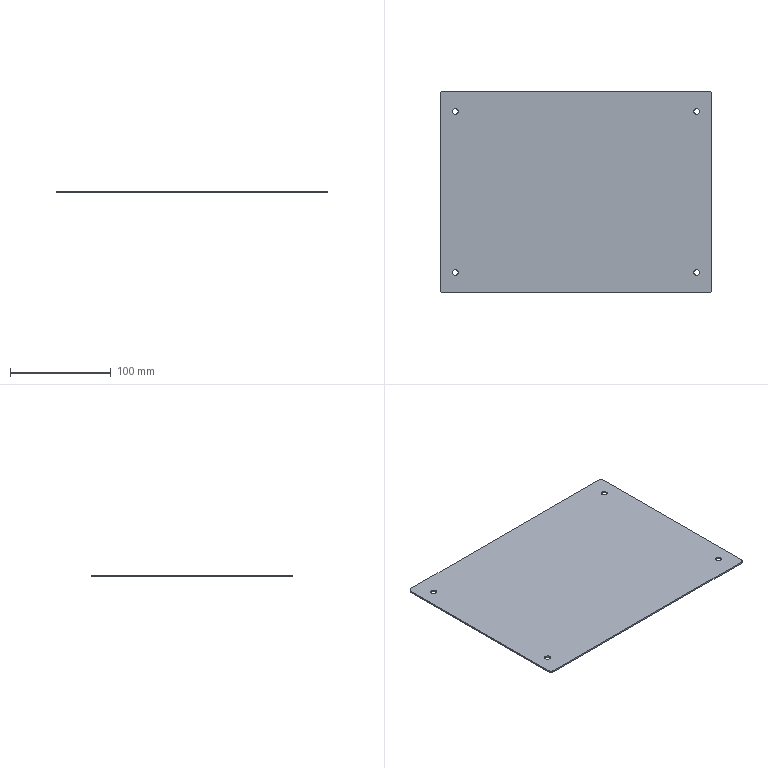Part | STEP file | J453-EBZ05-09-08-Part-1 | 1 solid | 18 faces | box 270 x 200 x 1.5 mm | volume 80830 mm3 | cylinder 12 | plane 6 | commonest cylinder face diameters 5.8 x8 6 x4